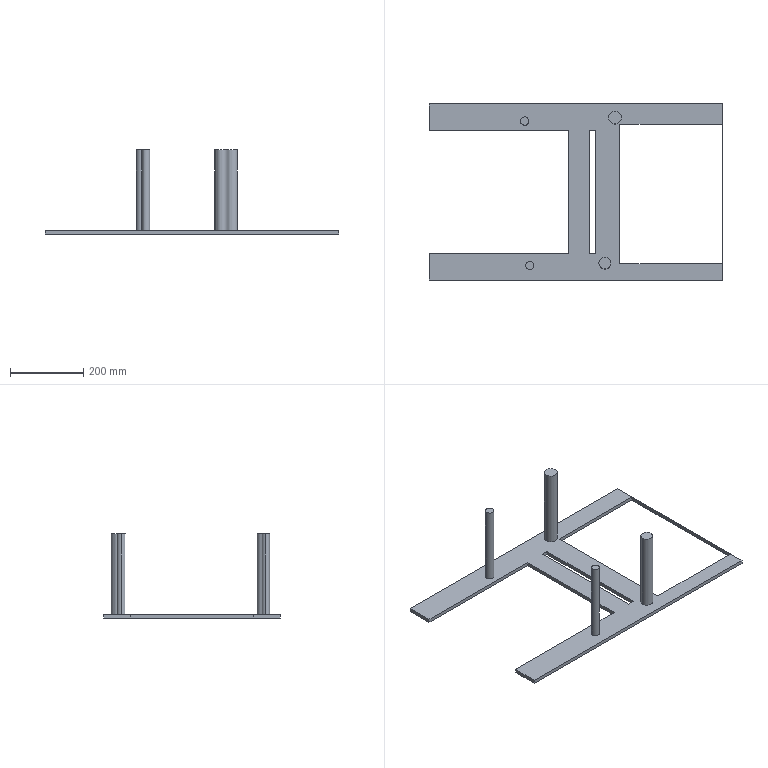Part | STEP file | 1 solid | 30 faces | box 800 x 480 x 230 mm | volume 2020030 mm3 | plane 22 | cylinder 8 | commonest cylinder face diameters 21.749 x2 22.904 x2 32.729 x2 35.198 x2